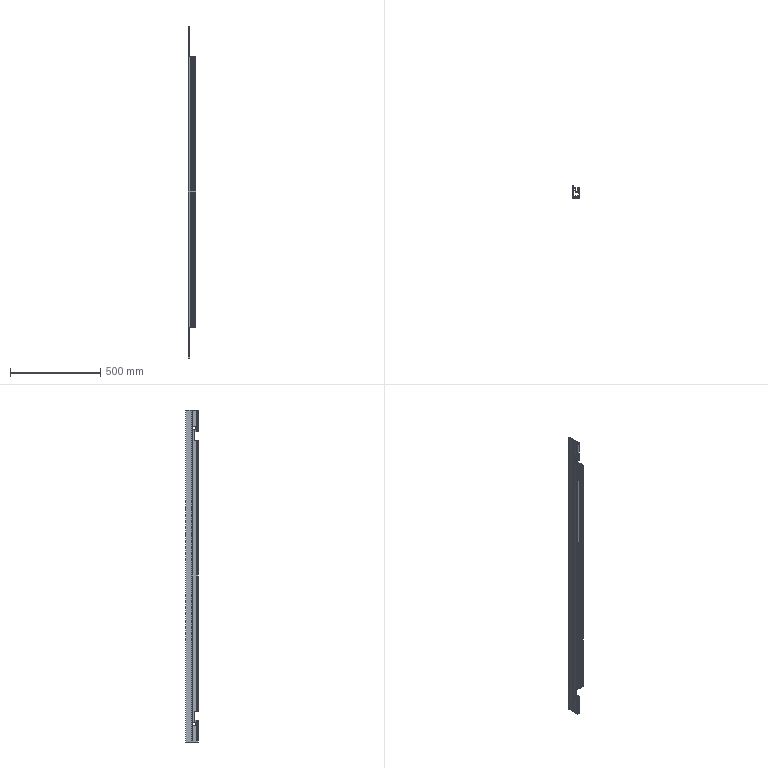Part | STEP file | MYT-A01-P02 | 1 solid | 234 faces | box 43 x 72 x 1840 mm | volume 1165090 mm3 | plane 156 | cylinder 78 | commonest cylinder face diameters 1 x70 22 x4 4 x2 2 x1 6.4 x1